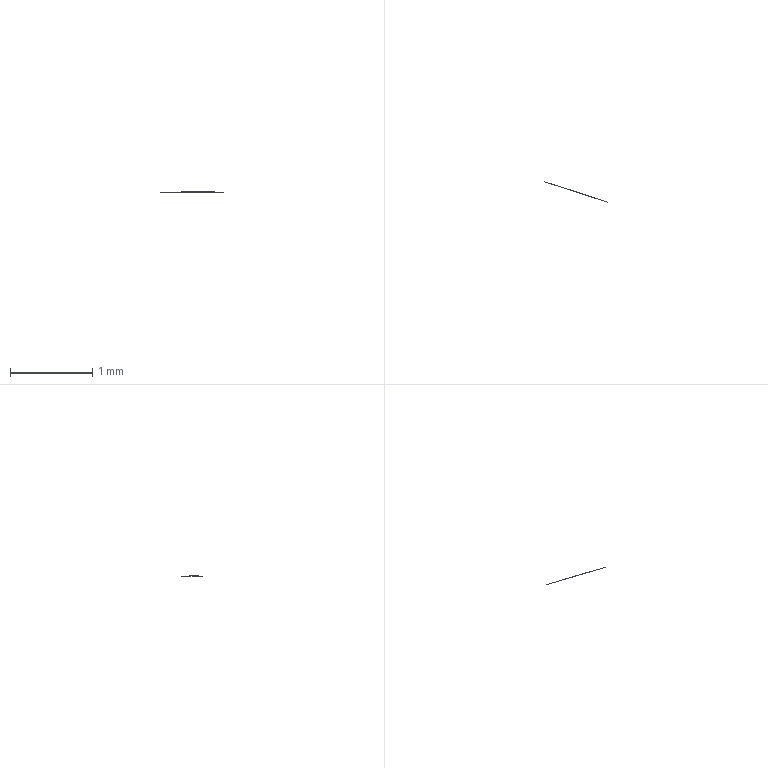Part | STEP file | 1_id290_x_t | 1 solid | 2 faces | box 4.043 x 0.7546 x 0.00007192 mm | volume 0.000006524 mm3 | torus 1 | spline 1